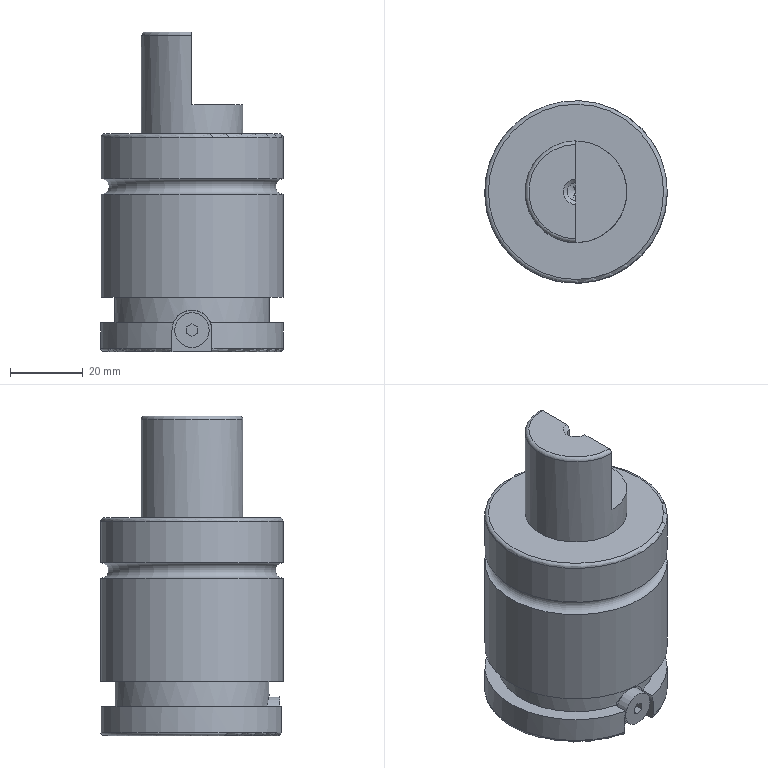Part | NX | features 24 2 | 1 solid | 173 faces | box 50.2 x 50.2 x 88 mm | volume 123875 mm3 | plane 130 | spline 25 | cylinder 10 | cone 4 | torus 4 | commonest cylinder face diameters 50.2 x3 6.6 x2 4.9 x1 9.5 x1 11 x1 28 x1